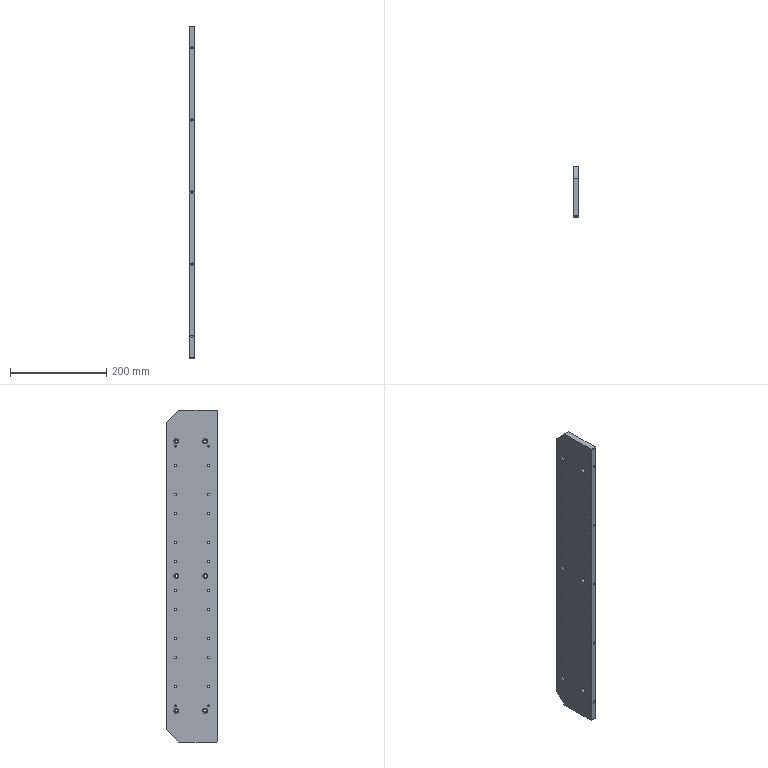Part | SolidWorks | features HoleWzd 4, Chamfer 2, Extrusion 1 | 1 solid | 128 faces | box 12 x 105 x 690 mm | volume 852566 mm3 | cylinder 92 | cone 20 | plane 16 | commonest cylinder face diameters 4.2 x48 5.5 x12 10 x12 2.5 x10 5 x10